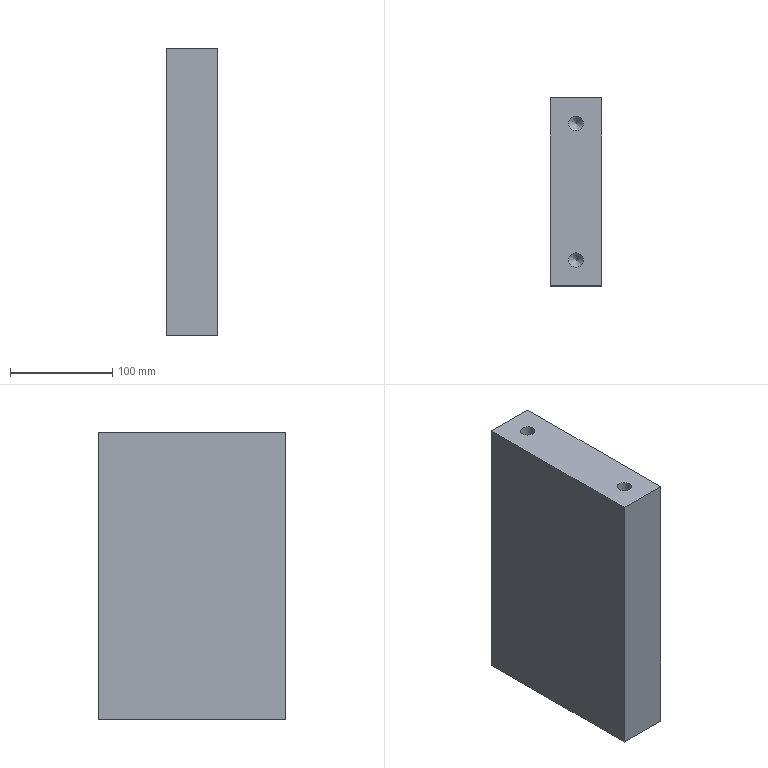Part | NX | features 29 2 | 1 solid | 14 faces | box 50 x 183.5 x 280.5 mm | volume 2549042 mm3 | plane 6 | cylinder 4 | cone 4 | commonest cylinder face diameters 14.1 x4
STEP:
#1=CARTESIAN_POINT('',(329.55,184.,-493.5));
#2=VERTEX_POINT('',#1);
#3=CARTESIAN_POINT('',(322.5,184.,-493.5));
#4=DIRECTION('',(0.,0.,1.));
#5=DIRECTION('',(1.,0.,0.));
#6=AXIS2_PLACEMENT_3D('',#3,#4,#5);
#7=CIRCLE('',#6,7.05);
#8=EDGE_CURVE('',#2,#2,#7,.T.);
#9=ORIENTED_EDGE('',*,*,#8,.T.);
#10=EDGE_LOOP('',(#9));
#11=FACE_BOUND('',#10,.T.);
#12=CARTESIAN_POINT('',(347.5,159.,-493.5));
#13=VERTEX_POINT('',#12);
#14=CARTESIAN_POINT('',(347.5,342.5,-493.5));
#15=VERTEX_POINT('',#14);
#16=CARTESIAN_POINT('',(347.5,193.,-493.5));
#17=DIRECTION('',(0.,1.,0.));
#18=VECTOR('',#17,1000.);
#19=LINE('',#16,#18);
#20=EDGE_CURVE('',#13,#15,#19,.T.);
#21=ORIENTED_EDGE('',*,*,#20,.F.);
#22=CARTESIAN_POINT('',(297.5,159.,-493.5));
#23=VERTEX_POINT('',#22);
#24=CARTESIAN_POINT('',(1915.,159.,-493.5));
#25=DIRECTION('',(-1.,0.,0.));
#26=VECTOR('',#25,1000.);
#27=LINE('',#24,#26);
#28=EDGE_CURVE('',#13,#23,#27,.T.);
#29=ORIENTED_EDGE('',*,*,#28,.T.);
#30=CARTESIAN_POINT('',(297.5,342.5,-493.5));
#31=VERTEX_POINT('',#30);
#32=CARTESIAN_POINT('',(297.5,193.,-493.5));
#33=DIRECTION('',(0.,-1.,0.));
#34=VECTOR('',#33,1000.);
#35=LINE('',#32,#34);
#36=EDGE_CURVE('',#31,#23,#35,.T.);
#37=ORIENTED_EDGE('',*,*,#36,.F.);
#38=CARTESIAN_POINT('',(242.5,342.5,-493.5));
#39=DIRECTION('',(1.,0.,0.));
#40=VECTOR('',#39,1000.);
#41=LINE('',#38,#40);
#42=EDGE_CURVE('',#31,#15,#41,.T.);
#43=ORIENTED_EDGE('',*,*,#42,.T.);
#44=EDGE_LOOP('',(#21,#29,#37,#43));
#45=FACE_BOUND('',#44,.T.);
#46=CARTESIAN_POINT('',(329.55,317.5,-493.5));
#47=VERTEX_POINT('',#46);
#48=CARTESIAN_POINT('',(322.5,317.5,-493.5));
#49=DIRECTION('',(0.,0.,1.));
#50=DIRECTION('',(1.,0.,0.));
#51=AXIS2_PLACEMENT_3D('',#48,#49,#50);
#52=CIRCLE('',#51,7.05);
#53=EDGE_CURVE('',#47,#47,#52,.T.);
#54=ORIENTED_EDGE('',*,*,#53,.T.);
#55=EDGE_LOOP('',(#54));
#56=FACE_BOUND('',#55,.T.);
#57=CARTESIAN_POINT('',(1915.,0.,-493.5));
#58=DIRECTION('',(0.,0.,-1.));
#59=DIRECTION('',(1.,0.,0.));
#60=AXIS2_PLACEMENT_3D('',#57,#58,#59);
#61=PLANE('',#60);
#62=ADVANCED_FACE('',(#11,#45,#56),#61,.T.);
#63=CARTESIAN_POINT('',(329.55,184.,-213.));
#64=VERTEX_POINT('',#63);
#65=CARTESIAN_POINT('',(322.5,184.,-213.));
#66=DIRECTION('',(0.,0.,-1.));
#67=DIRECTION('',(1.,0.,0.));
#68=AXIS2_PLACEMENT_3D('',#65,#66,#67);
#69=CIRCLE('',#68,7.05);
#70=EDGE_CURVE('',#64,#64,#69,.T.);
#71=ORIENTED_EDGE('',*,*,#70,.T.);
#72=EDGE_LOOP('',(#71));
#73=FACE_BOUND('',#72,.T.);
#74=CARTESIAN_POINT('',(297.5,159.,-213.));
#75=VERTEX_POINT('',#74);
#76=CARTESIAN_POINT('',(297.5,342.5,-213.));
#77=VERTEX_POINT('',#76);
#78=CARTESIAN_POINT('',(297.5,193.,-213.));
#79=DIRECTION('',(0.,1.,0.));
#80=VECTOR('',#79,1000.);
#81=LINE('',#78,#80);
#82=EDGE_CURVE('',#75,#77,#81,.T.);
#83=ORIENTED_EDGE('',*,*,#82,.F.);
#84=CARTESIAN_POINT('',(347.5,159.,-213.));
#85=VERTEX_POINT('',#84);
#86=CARTESIAN_POINT('',(1915.,159.,-213.));
#87=DIRECTION('',(1.,0.,0.));
#88=VECTOR('',#87,1000.);
#89=LINE('',#86,#88);
#90=EDGE_CURVE('',#75,#85,#89,.T.);
#91=ORIENTED_EDGE('',*,*,#90,.T.);
#92=CARTESIAN_POINT('',(347.5,342.5,-213.));
#93=VERTEX_POINT('',#92);
#94=CARTESIAN_POINT('',(347.5,193.,-213.));
#95=DIRECTION('',(0.,-1.,0.));
#96=VECTOR('',#95,1000.);
#97=LINE('',#94,#96);
#98=EDGE_CURVE('',#93,#85,#97,.T.);
#99=ORIENTED_EDGE('',*,*,#98,.F.);
#100=CARTESIAN_POINT('',(242.5,342.5,-213.));
#101=DIRECTION('',(-1.,0.,0.));
#102=VECTOR('',#101,1000.);
#103=LINE('',#100,#102);
#104=EDGE_CURVE('',#93,#77,#103,.T.);
#105=ORIENTED_EDGE('',*,*,#104,.T.);
#106=EDGE_LOOP('',(#83,#91,#99,#105));
#107=FACE_BOUND('',#106,.T.);
#108=CARTESIAN_POINT('',(329.55,317.5,-213.));
#109=VERTEX_POINT('',#108);
#110=CARTESIAN_POINT('',(322.5,317.5,-213.));
#111=DIRECTION('',(0.,0.,-1.));
#112=DIRECTION('',(1.,0.,0.));
#113=AXIS2_PLACEMENT_3D('',#110,#111,#112);
#114=CIRCLE('',#113,7.05);
#115=EDGE_CURVE('',#109,#109,#114,.T.);
#116=ORIENTED_EDGE('',*,*,#115,.T.);
#117=EDGE_LOOP('',(#116));
#118=FACE_BOUND('',#117,.T.);
#119=CARTESIAN_POINT('',(1915.,0.,-213.));
#120=DIRECTION('',(0.,0.,1.));
#121=DIRECTION('',(-1.,0.,0.));
#122=AXIS2_PLACEMENT_3D('',#119,#120,#121);
#123=PLANE('',#122);
#124=ADVANCED_FACE('',(#73,#107,#118),#123,.T.);
#125=ORIENTED_EDGE('',*,*,#90,.F.);
#126=CARTESIAN_POINT('',(297.5,159.,-205.5));
#127=DIRECTION('',(0.,0.,1.));
#128=VECTOR('',#127,1000.);
#129=LINE('',#126,#128);
#130=EDGE_CURVE('',#23,#75,#129,.T.);
#131=ORIENTED_EDGE('',*,*,#130,.F.);
#132=ORIENTED_EDGE('',*,*,#28,.F.);
#133=CARTESIAN_POINT('',(347.5,159.,-205.5));
#134=DIRECTION('',(0.,0.,-1.));
#135=VECTOR('',#134,1000.);
#136=LINE('',#133,#135);
#137=EDGE_CURVE('',#85,#13,#136,.T.);
#138=ORIENTED_EDGE('',*,*,#137,.F.);
#139=EDGE_LOOP('',(#125,#131,#132,#138));
#140=FACE_BOUND('',#139,.T.);
#141=CARTESIAN_POINT('',(210.,159.,0.));
#142=DIRECTION('',(0.,-1.,0.));
#143=DIRECTION('',(0.,0.,1.));
#144=AXIS2_PLACEMENT_3D('',#141,#142,#143);
#145=PLANE('',#144);
#146=ADVANCED_FACE('',(#140),#145,.T.);
#147=ORIENTED_EDGE('',*,*,#36,.T.);
#148=ORIENTED_EDGE('',*,*,#130,.T.);
#149=ORIENTED_EDGE('',*,*,#82,.T.);
#150=CARTESIAN_POINT('',(297.5,342.5,-205.5));
#151=DIRECTION('',(0.,0.,1.));
#152=VECTOR('',#151,1000.);
#153=LINE('',#150,#152);
#154=EDGE_CURVE('',#31,#77,#153,.T.);
#155=ORIENTED_EDGE('',*,*,#154,.F.);
#156=EDGE_LOOP('',(#147,#148,#149,#155));
#157=FACE_BOUND('',#156,.T.);
#158=CARTESIAN_POINT('',(297.5,193.,-205.5));
#159=DIRECTION('',(-1.,0.,0.));
#160=DIRECTION('',(0.,0.,1.));
#161=AXIS2_PLACEMENT_3D('',#158,#159,#160);
#162=PLANE('',#161);
#163=ADVANCED_FACE('',(#157),#162,.T.);
#164=ORIENTED_EDGE('',*,*,#98,.T.);
#165=ORIENTED_EDGE('',*,*,#137,.T.);
#166=ORIENTED_EDGE('',*,*,#20,.T.);
#167=CARTESIAN_POINT('',(347.5,342.5,91.));
#168=DIRECTION('',(0.,0.,1.));
#169=VECTOR('',#168,1000.);
#170=LINE('',#167,#169);
#171=EDGE_CURVE('',#15,#93,#170,.T.);
#172=ORIENTED_EDGE('',*,*,#171,.T.);
#173=EDGE_LOOP('',(#164,#165,#166,#172));
#174=FACE_BOUND('',#173,.T.);
#175=CARTESIAN_POINT('',(347.5,193.,-205.5));
#176=DIRECTION('',(1.,0.,0.));
#177=DIRECTION('',(0.,0.,-1.));
#178=AXIS2_PLACEMENT_3D('',#175,#176,#177);
#179=PLANE('',#178);
#180=ADVANCED_FACE('',(#174),#179,.T.);
#181=ORIENTED_EDGE('',*,*,#42,.F.);
#182=ORIENTED_EDGE('',*,*,#154,.T.);
#183=ORIENTED_EDGE('',*,*,#104,.F.);
#184=ORIENTED_EDGE('',*,*,#171,.F.);
#185=EDGE_LOOP('',(#181,#182,#183,#184));
#186=FACE_BOUND('',#185,.T.);
#187=CARTESIAN_POINT('',(242.5,342.5,91.));
#188=DIRECTION('',(0.,-1.,0.));
#189=DIRECTION('',(-1.,0.,0.));
#190=AXIS2_PLACEMENT_3D('',#187,#188,#189);
#191=PLANE('',#190);
#192=ADVANCED_FACE('',(#186),#191,.F.);
#193=CARTESIAN_POINT('',(315.45,184.,-249.95));
#194=VERTEX_POINT('',#193);
#195=CARTESIAN_POINT('',(322.5,184.,-249.95));
#196=DIRECTION('',(0.,0.,-1.));
#197=DIRECTION('',(-1.,0.,0.));
#198=AXIS2_PLACEMENT_3D('',#195,#196,#197);
#199=CIRCLE('',#198,7.05);
#200=EDGE_CURVE('',#194,#194,#199,.T.);
#201=ORIENTED_EDGE('',*,*,#200,.T.);
#202=EDGE_LOOP('',(#201));
#203=FACE_BOUND('',#202,.T.);
#204=ORIENTED_EDGE('',*,*,#70,.F.);
#205=EDGE_LOOP('',(#204));
#206=FACE_BOUND('',#205,.T.);
#207=CARTESIAN_POINT('',(322.5,184.,-213.));
#208=DIRECTION('',(0.,0.,-1.));
#209=DIRECTION('',(-1.,0.,0.));
#210=AXIS2_PLACEMENT_3D('',#207,#208,#209);
#211=CYLINDRICAL_SURFACE('',#210,7.05);
#212=ADVANCED_FACE('',(#203,#206),#211,.F.);
#213=CARTESIAN_POINT('',(322.5,184.,-257.));
#214=VERTEX_POINT('',#213);
#215=VERTEX_LOOP('',#214);
#216=FACE_BOUND('',#215,.T.);
#217=ORIENTED_EDGE('',*,*,#200,.F.);
#218=EDGE_LOOP('',(#217));
#219=FACE_BOUND('',#218,.T.);
#220=CARTESIAN_POINT('',(322.5,184.,-249.95));
#221=DIRECTION('',(0.,0.,1.));
#222=DIRECTION('',(-1.,0.,0.));
#223=AXIS2_PLACEMENT_3D('',#220,#221,#222);
#224=CONICAL_SURFACE('',#223,7.05,0.7854);
#225=ADVANCED_FACE('',(#216,#219),#224,.F.);
#226=CARTESIAN_POINT('',(315.45,317.5,-249.95));
#227=VERTEX_POINT('',#226);
#228=CARTESIAN_POINT('',(322.5,317.5,-249.95));
#229=DIRECTION('',(0.,0.,-1.));
#230=DIRECTION('',(-1.,0.,0.));
#231=AXIS2_PLACEMENT_3D('',#228,#229,#230);
#232=CIRCLE('',#231,7.05);
#233=EDGE_CURVE('',#227,#227,#232,.T.);
#234=ORIENTED_EDGE('',*,*,#233,.T.);
#235=EDGE_LOOP('',(#234));
#236=FACE_BOUND('',#235,.T.);
#237=ORIENTED_EDGE('',*,*,#115,.F.);
#238=EDGE_LOOP('',(#237));
#239=FACE_BOUND('',#238,.T.);
#240=CARTESIAN_POINT('',(322.5,317.5,-213.));
#241=DIRECTION('',(0.,0.,-1.));
#242=DIRECTION('',(-1.,0.,0.));
#243=AXIS2_PLACEMENT_3D('',#240,#241,#242);
#244=CYLINDRICAL_SURFACE('',#243,7.05);
#245=ADVANCED_FACE('',(#236,#239),#244,.F.);
#246=CARTESIAN_POINT('',(322.5,317.5,-257.));
#247=VERTEX_POINT('',#246);
#248=VERTEX_LOOP('',#247);
#249=FACE_BOUND('',#248,.T.);
#250=ORIENTED_EDGE('',*,*,#233,.F.);
#251=EDGE_LOOP('',(#250));
#252=FACE_BOUND('',#251,.T.);
#253=CARTESIAN_POINT('',(322.5,317.5,-249.95));
#254=DIRECTION('',(0.,0.,1.));
#255=DIRECTION('',(-1.,0.,0.));
#256=AXIS2_PLACEMENT_3D('',#253,#254,#255);
#257=CONICAL_SURFACE('',#256,7.05,0.7854);
#258=ADVANCED_FACE('',(#249,#252),#257,.F.);
#259=CARTESIAN_POINT('',(329.55,184.,-456.55));
#260=VERTEX_POINT('',#259);
#261=CARTESIAN_POINT('',(322.5,184.,-456.55));
#262=DIRECTION('',(0.,0.,1.));
#263=DIRECTION('',(1.,0.,0.));
#264=AXIS2_PLACEMENT_3D('',#261,#262,#263);
#265=CIRCLE('',#264,7.05);
#266=EDGE_CURVE('',#260,#260,#265,.T.);
#267=ORIENTED_EDGE('',*,*,#266,.T.);
#268=EDGE_LOOP('',(#267));
#269=FACE_BOUND('',#268,.T.);
#270=ORIENTED_EDGE('',*,*,#8,.F.);
#271=EDGE_LOOP('',(#270));
#272=FACE_BOUND('',#271,.T.);
#273=CARTESIAN_POINT('',(322.5,184.,-493.5));
#274=DIRECTION('',(0.,0.,1.));
#275=DIRECTION('',(-1.,0.,0.));
#276=AXIS2_PLACEMENT_3D('',#273,#274,#275);
#277=CYLINDRICAL_SURFACE('',#276,7.05);
#278=ADVANCED_FACE('',(#269,#272),#277,.F.);
#279=CARTESIAN_POINT('',(322.5,184.,-449.5));
#280=VERTEX_POINT('',#279);
#281=VERTEX_LOOP('',#280);
#282=FACE_BOUND('',#281,.T.);
#283=ORIENTED_EDGE('',*,*,#266,.F.);
#284=EDGE_LOOP('',(#283));
#285=FACE_BOUND('',#284,.T.);
#286=CARTESIAN_POINT('',(322.5,184.,-456.55));
#287=DIRECTION('',(0.,0.,-1.));
#288=DIRECTION('',(1.,0.,0.));
#289=AXIS2_PLACEMENT_3D('',#286,#287,#288);
#290=CONICAL_SURFACE('',#289,7.05,0.7854);
#291=ADVANCED_FACE('',(#282,#285),#290,.F.);
#292=CARTESIAN_POINT('',(329.55,317.5,-456.55));
#293=VERTEX_POINT('',#292);
#294=CARTESIAN_POINT('',(322.5,317.5,-456.55));
#295=DIRECTION('',(0.,0.,1.));
#296=DIRECTION('',(1.,0.,0.));
#297=AXIS2_PLACEMENT_3D('',#294,#295,#296);
#298=CIRCLE('',#297,7.05);
#299=EDGE_CURVE('',#293,#293,#298,.T.);
#300=ORIENTED_EDGE('',*,*,#299,.T.);
#301=EDGE_LOOP('',(#300));
#302=FACE_BOUND('',#301,.T.);
#303=ORIENTED_EDGE('',*,*,#53,.F.);
#304=EDGE_LOOP('',(#303));
#305=FACE_BOUND('',#304,.T.);
#306=CARTESIAN_POINT('',(322.5,317.5,-493.5));
#307=DIRECTION('',(0.,0.,1.));
#308=DIRECTION('',(-1.,0.,0.));
#309=AXIS2_PLACEMENT_3D('',#306,#307,#308);
#310=CYLINDRICAL_SURFACE('',#309,7.05);
#311=ADVANCED_FACE('',(#302,#305),#310,.F.);
#312=CARTESIAN_POINT('',(322.5,317.5,-449.5));
#313=VERTEX_POINT('',#312);
#314=VERTEX_LOOP('',#313);
#315=FACE_BOUND('',#314,.T.);
#316=ORIENTED_EDGE('',*,*,#299,.F.);
#317=EDGE_LOOP('',(#316));
#318=FACE_BOUND('',#317,.T.);
#319=CARTESIAN_POINT('',(322.5,317.5,-456.55));
#320=DIRECTION('',(0.,0.,-1.));
#321=DIRECTION('',(1.,0.,0.));
#322=AXIS2_PLACEMENT_3D('',#319,#320,#321);
#323=CONICAL_SURFACE('',#322,7.05,0.7854);
#324=ADVANCED_FACE('',(#315,#318),#323,.F.);
#325=CLOSED_SHELL('',(#62,#124,#146,#163,#180,#192,#212,#225,#245,#258,#278,#291,#311,#324));
#326=MANIFOLD_SOLID_BREP('',#325);
#327=(LENGTH_UNIT()NAMED_UNIT(*)SI_UNIT(.MILLI.,.METRE.));
#328=UNCERTAINTY_MEASURE_WITH_UNIT(LENGTH_MEASURE(0.00001),#327,'','');
#329=(NAMED_UNIT(*)PLANE_ANGLE_UNIT()SI_UNIT($,.RADIAN.));
#330=(NAMED_UNIT(*)SI_UNIT($,.STERADIAN.)SOLID_ANGLE_UNIT());
#331=(GEOMETRIC_REPRESENTATION_CONTEXT(3)GLOBAL_UNCERTAINTY_ASSIGNED_CONTEXT((#328))GLOBAL_UNIT_ASSIGNED_CONTEXT((#327,#329,#330))REPRESENTATION_CONTEXT('',''));
#332=ADVANCED_BREP_SHAPE_REPRESENTATION('',(#326),#331);